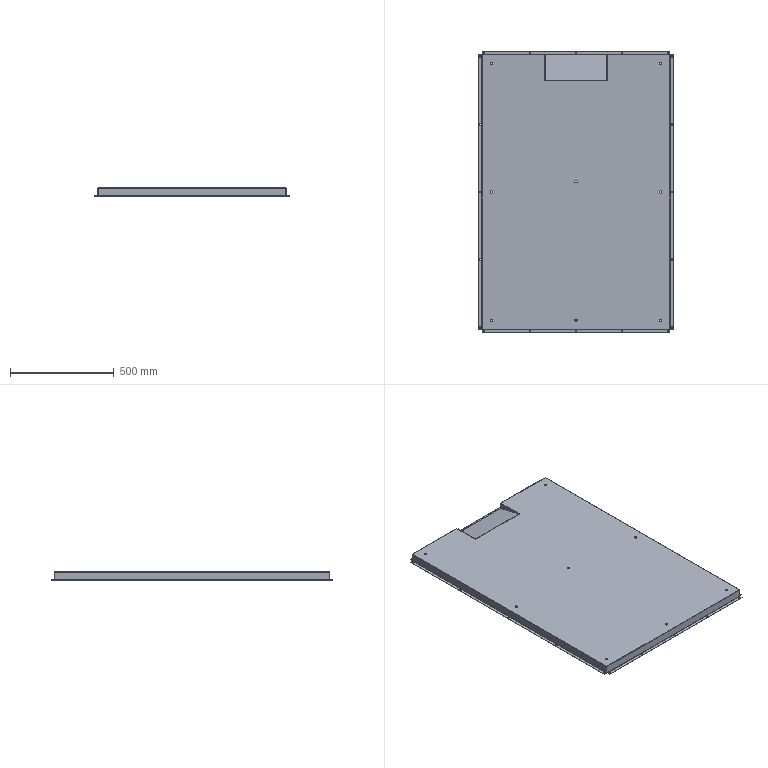Part | SolidWorks | 2 solids | 206 faces | box 939 x 1359 x 40 mm | volume 1439587 mm3 | plane 106 | cylinder 88 | spline 12 | commonest cylinder face diameters 7 x50 11 x16 0.4 x11 2.4 x11